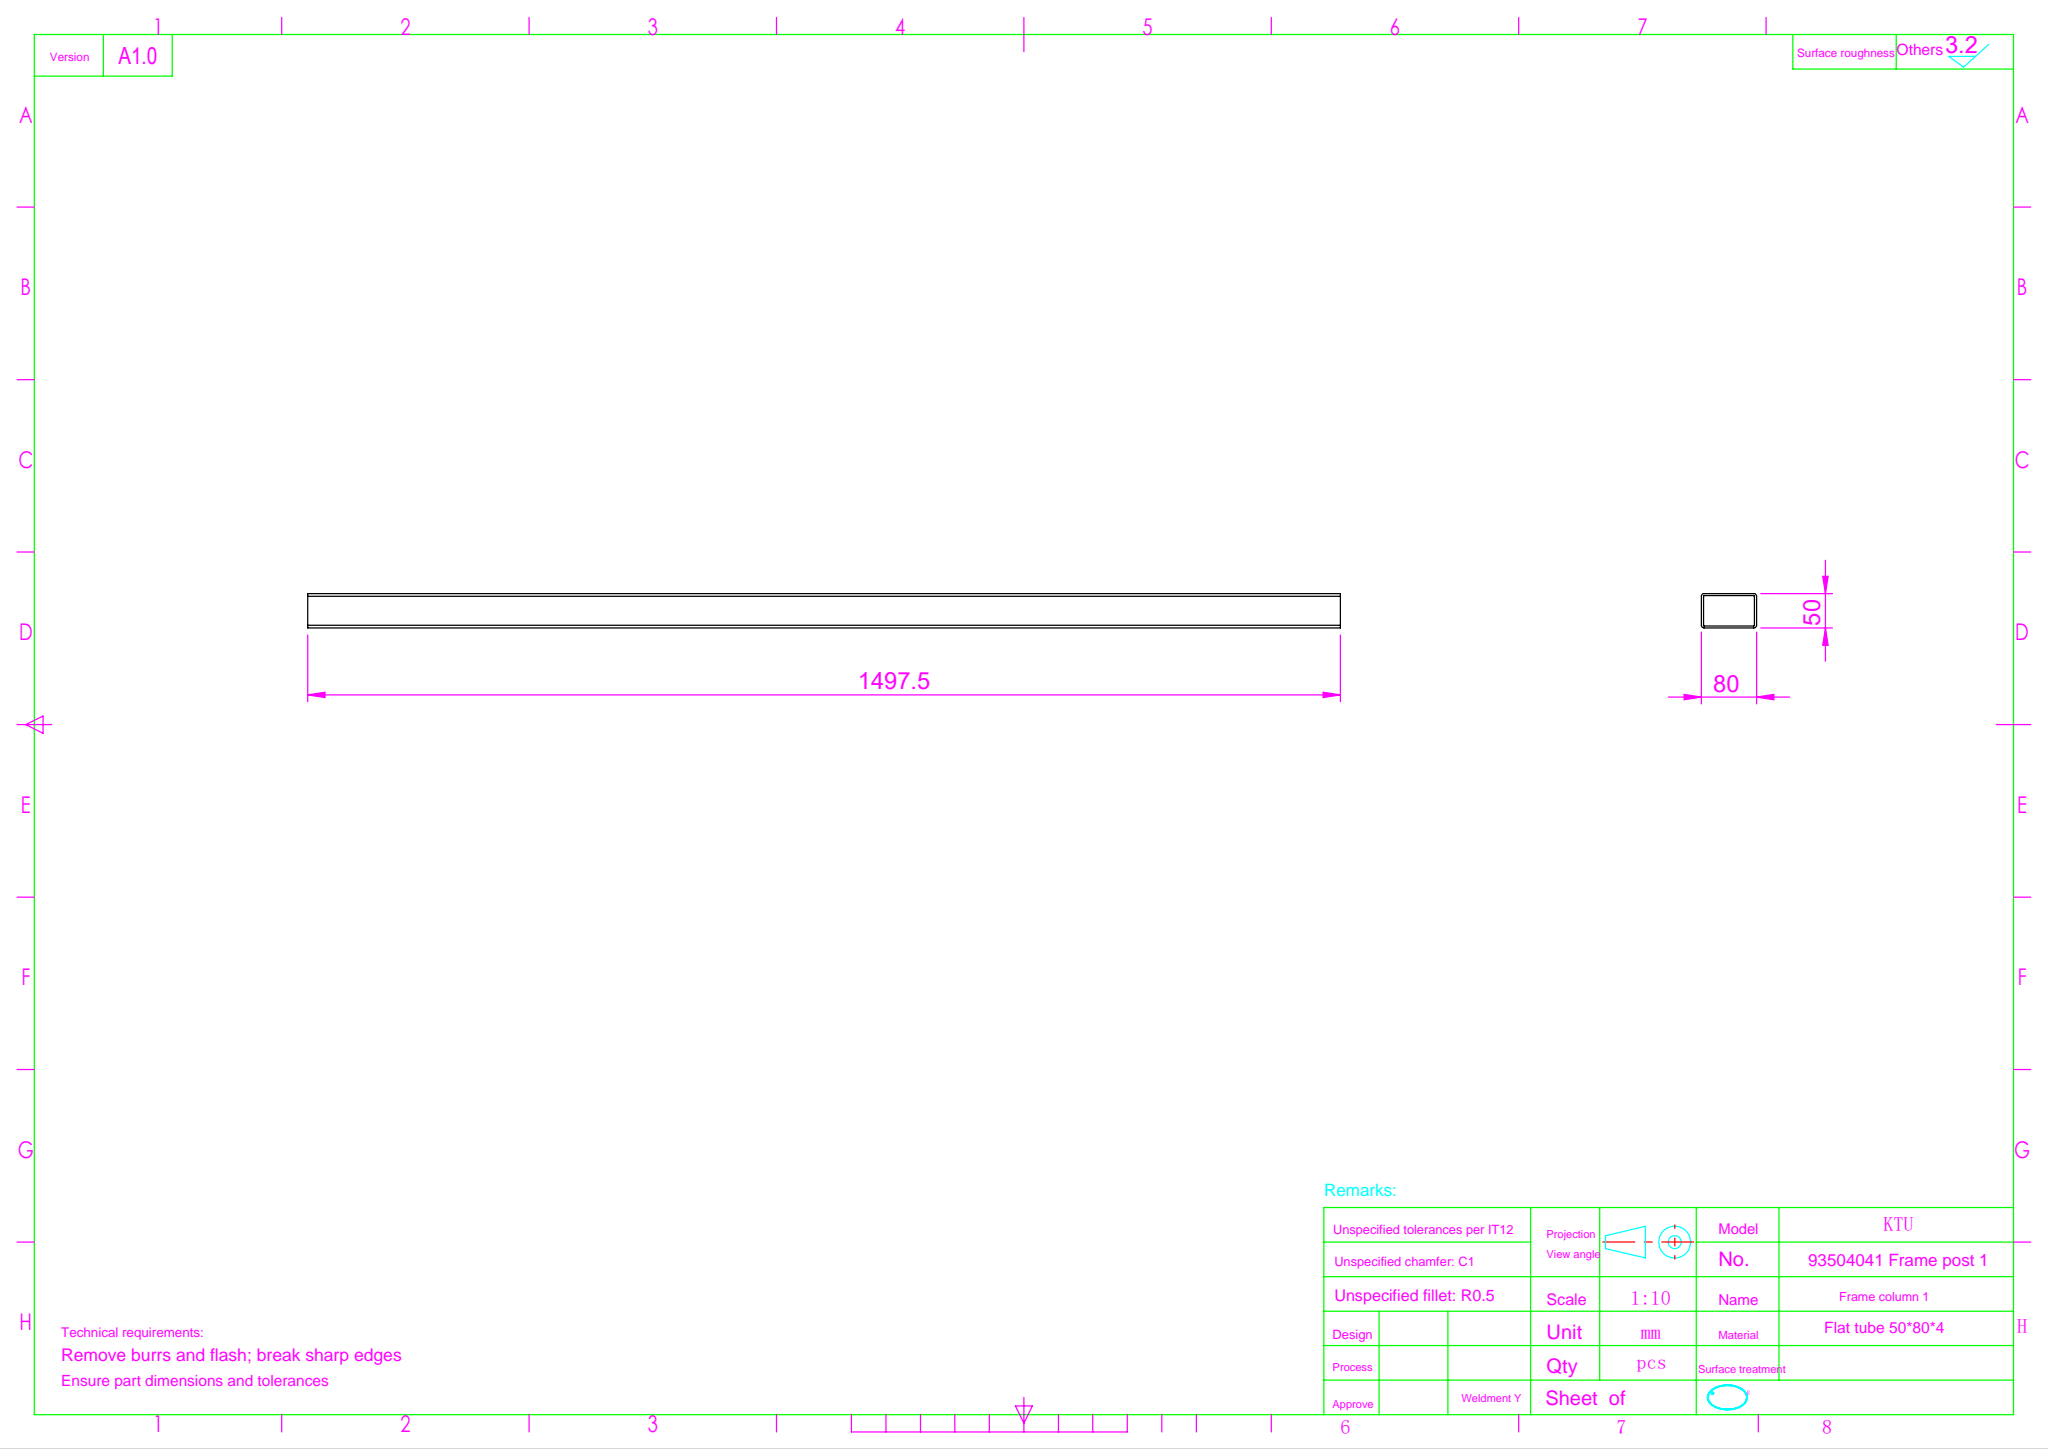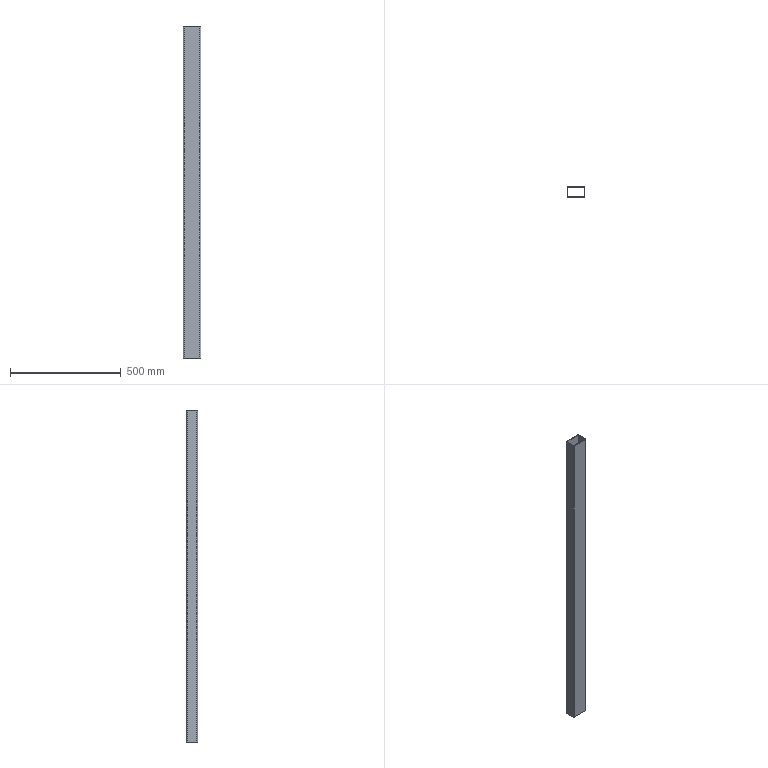Part | SolidWorks | features ExtruThin 1 | 1 solid | 18 faces | box 80 x 50 x 1498 mm | volume 1094858 mm3 | plane 10 | cylinder 8 | commonest cylinder face diameters 2 x4 8 x4
STEP:
#1=CARTESIAN_POINT('',(36.,-25.,748.75));
#2=VERTEX_POINT('',#1);
#3=CARTESIAN_POINT('',(40.,-21.,748.75));
#4=VERTEX_POINT('',#3);
#5=CARTESIAN_POINT('',(36.,-21.,748.75));
#6=DIRECTION('',(0.,0.,1.));
#7=DIRECTION('',(1.,0.,0.));
#8=AXIS2_PLACEMENT_3D('',#5,#6,#7);
#9=CIRCLE('',#8,4.);
#10=EDGE_CURVE('',#2,#4,#9,.T.);
#11=ORIENTED_EDGE('',*,*,#10,.T.);
#12=CARTESIAN_POINT('',(40.,21.,748.75));
#13=VERTEX_POINT('',#12);
#14=CARTESIAN_POINT('',(40.,21.,748.75));
#15=DIRECTION('',(0.,1.,0.));
#16=VECTOR('',#15,1000.);
#17=LINE('',#14,#16);
#18=EDGE_CURVE('',#4,#13,#17,.T.);
#19=ORIENTED_EDGE('',*,*,#18,.T.);
#20=CARTESIAN_POINT('',(36.,25.,748.75));
#21=VERTEX_POINT('',#20);
#22=CARTESIAN_POINT('',(36.,21.,748.75));
#23=DIRECTION('',(0.,0.,1.));
#24=DIRECTION('',(-1.,0.,0.));
#25=AXIS2_PLACEMENT_3D('',#22,#23,#24);
#26=CIRCLE('',#25,4.);
#27=EDGE_CURVE('',#13,#21,#26,.T.);
#28=ORIENTED_EDGE('',*,*,#27,.T.);
#29=CARTESIAN_POINT('',(-36.,25.,748.75));
#30=VERTEX_POINT('',#29);
#31=CARTESIAN_POINT('',(-36.,25.,748.75));
#32=DIRECTION('',(-1.,0.,0.));
#33=VECTOR('',#32,1000.);
#34=LINE('',#31,#33);
#35=EDGE_CURVE('',#21,#30,#34,.T.);
#36=ORIENTED_EDGE('',*,*,#35,.T.);
#37=CARTESIAN_POINT('',(-40.,21.,748.75));
#38=VERTEX_POINT('',#37);
#39=CARTESIAN_POINT('',(-36.,21.,748.75));
#40=DIRECTION('',(0.,0.,1.));
#41=DIRECTION('',(1.,0.,0.));
#42=AXIS2_PLACEMENT_3D('',#39,#40,#41);
#43=CIRCLE('',#42,4.);
#44=EDGE_CURVE('',#30,#38,#43,.T.);
#45=ORIENTED_EDGE('',*,*,#44,.T.);
#46=CARTESIAN_POINT('',(-40.,-21.,748.75));
#47=VERTEX_POINT('',#46);
#48=CARTESIAN_POINT('',(-40.,21.,748.75));
#49=DIRECTION('',(0.,-1.,0.));
#50=VECTOR('',#49,1000.);
#51=LINE('',#48,#50);
#52=EDGE_CURVE('',#38,#47,#51,.T.);
#53=ORIENTED_EDGE('',*,*,#52,.T.);
#54=CARTESIAN_POINT('',(-36.,-25.,748.75));
#55=VERTEX_POINT('',#54);
#56=CARTESIAN_POINT('',(-36.,-21.,748.75));
#57=DIRECTION('',(0.,0.,1.));
#58=DIRECTION('',(1.,0.,0.));
#59=AXIS2_PLACEMENT_3D('',#56,#57,#58);
#60=CIRCLE('',#59,4.);
#61=EDGE_CURVE('',#47,#55,#60,.T.);
#62=ORIENTED_EDGE('',*,*,#61,.T.);
#63=CARTESIAN_POINT('',(-36.,-25.,748.75));
#64=DIRECTION('',(1.,0.,0.));
#65=VECTOR('',#64,1000.);
#66=LINE('',#63,#65);
#67=EDGE_CURVE('',#55,#2,#66,.T.);
#68=ORIENTED_EDGE('',*,*,#67,.T.);
#69=EDGE_LOOP('',(#11,#19,#28,#36,#45,#53,#62,#68));
#70=FACE_OUTER_BOUND('',#69,.T.);
#71=CARTESIAN_POINT('',(37.,-21.,748.75));
#72=VERTEX_POINT('',#71);
#73=CARTESIAN_POINT('',(37.,21.,748.75));
#74=VERTEX_POINT('',#73);
#75=CARTESIAN_POINT('',(37.,21.,748.75));
#76=DIRECTION('',(0.,1.,0.));
#77=VECTOR('',#76,1000.);
#78=LINE('',#75,#77);
#79=EDGE_CURVE('',#72,#74,#78,.T.);
#80=ORIENTED_EDGE('',*,*,#79,.F.);
#81=CARTESIAN_POINT('',(36.,-22.,748.75));
#82=VERTEX_POINT('',#81);
#83=CARTESIAN_POINT('',(36.,-21.,748.75));
#84=DIRECTION('',(0.,0.,1.));
#85=DIRECTION('',(1.,0.,0.));
#86=AXIS2_PLACEMENT_3D('',#83,#84,#85);
#87=CIRCLE('',#86,1.);
#88=EDGE_CURVE('',#82,#72,#87,.T.);
#89=ORIENTED_EDGE('',*,*,#88,.F.);
#90=CARTESIAN_POINT('',(-36.,-22.,748.75));
#91=VERTEX_POINT('',#90);
#92=CARTESIAN_POINT('',(-36.,-22.,748.75));
#93=DIRECTION('',(1.,0.,0.));
#94=VECTOR('',#93,1000.);
#95=LINE('',#92,#94);
#96=EDGE_CURVE('',#91,#82,#95,.T.);
#97=ORIENTED_EDGE('',*,*,#96,.F.);
#98=CARTESIAN_POINT('',(-37.,-21.,748.75));
#99=VERTEX_POINT('',#98);
#100=CARTESIAN_POINT('',(-36.,-21.,748.75));
#101=DIRECTION('',(0.,0.,1.));
#102=DIRECTION('',(1.,0.,0.));
#103=AXIS2_PLACEMENT_3D('',#100,#101,#102);
#104=CIRCLE('',#103,1.);
#105=EDGE_CURVE('',#99,#91,#104,.T.);
#106=ORIENTED_EDGE('',*,*,#105,.F.);
#107=CARTESIAN_POINT('',(-37.,21.,748.75));
#108=VERTEX_POINT('',#107);
#109=CARTESIAN_POINT('',(-37.,21.,748.75));
#110=DIRECTION('',(0.,-1.,0.));
#111=VECTOR('',#110,1000.);
#112=LINE('',#109,#111);
#113=EDGE_CURVE('',#108,#99,#112,.T.);
#114=ORIENTED_EDGE('',*,*,#113,.F.);
#115=CARTESIAN_POINT('',(-36.,22.,748.75));
#116=VERTEX_POINT('',#115);
#117=CARTESIAN_POINT('',(-36.,21.,748.75));
#118=DIRECTION('',(0.,0.,1.));
#119=DIRECTION('',(1.,0.,0.));
#120=AXIS2_PLACEMENT_3D('',#117,#118,#119);
#121=CIRCLE('',#120,1.);
#122=EDGE_CURVE('',#116,#108,#121,.T.);
#123=ORIENTED_EDGE('',*,*,#122,.F.);
#124=CARTESIAN_POINT('',(36.,22.,748.75));
#125=VERTEX_POINT('',#124);
#126=CARTESIAN_POINT('',(-36.,22.,748.75));
#127=DIRECTION('',(-1.,0.,0.));
#128=VECTOR('',#127,1000.);
#129=LINE('',#126,#128);
#130=EDGE_CURVE('',#125,#116,#129,.T.);
#131=ORIENTED_EDGE('',*,*,#130,.F.);
#132=CARTESIAN_POINT('',(36.,21.,748.75));
#133=DIRECTION('',(0.,0.,1.));
#134=DIRECTION('',(1.,0.,0.));
#135=AXIS2_PLACEMENT_3D('',#132,#133,#134);
#136=CIRCLE('',#135,1.);
#137=EDGE_CURVE('',#74,#125,#136,.T.);
#138=ORIENTED_EDGE('',*,*,#137,.F.);
#139=EDGE_LOOP('',(#80,#89,#97,#106,#114,#123,#131,#138));
#140=FACE_BOUND('',#139,.T.);
#141=CARTESIAN_POINT('',(36.,-21.,748.75));
#142=DIRECTION('',(0.,0.,1.));
#143=DIRECTION('',(1.,0.,0.));
#144=AXIS2_PLACEMENT_3D('',#141,#142,#143);
#145=PLANE('',#144);
#146=ADVANCED_FACE('',(#70,#140),#145,.T.);
#147=CARTESIAN_POINT('',(36.,-25.,-748.75));
#148=VERTEX_POINT('',#147);
#149=CARTESIAN_POINT('',(40.,-21.,-748.75));
#150=VERTEX_POINT('',#149);
#151=CARTESIAN_POINT('',(36.,-21.,-748.75));
#152=DIRECTION('',(0.,0.,1.));
#153=DIRECTION('',(1.,0.,0.));
#154=AXIS2_PLACEMENT_3D('',#151,#152,#153);
#155=CIRCLE('',#154,4.);
#156=EDGE_CURVE('',#148,#150,#155,.T.);
#157=ORIENTED_EDGE('',*,*,#156,.F.);
#158=CARTESIAN_POINT('',(-36.,-25.,-748.75));
#159=VERTEX_POINT('',#158);
#160=CARTESIAN_POINT('',(-36.,-25.,-748.75));
#161=DIRECTION('',(1.,0.,0.));
#162=VECTOR('',#161,1000.);
#163=LINE('',#160,#162);
#164=EDGE_CURVE('',#159,#148,#163,.T.);
#165=ORIENTED_EDGE('',*,*,#164,.F.);
#166=CARTESIAN_POINT('',(-40.,-21.,-748.75));
#167=VERTEX_POINT('',#166);
#168=CARTESIAN_POINT('',(-36.,-21.,-748.75));
#169=DIRECTION('',(0.,0.,1.));
#170=DIRECTION('',(1.,0.,0.));
#171=AXIS2_PLACEMENT_3D('',#168,#169,#170);
#172=CIRCLE('',#171,4.);
#173=EDGE_CURVE('',#167,#159,#172,.T.);
#174=ORIENTED_EDGE('',*,*,#173,.F.);
#175=CARTESIAN_POINT('',(-40.,21.,-748.75));
#176=VERTEX_POINT('',#175);
#177=CARTESIAN_POINT('',(-40.,21.,-748.75));
#178=DIRECTION('',(0.,-1.,0.));
#179=VECTOR('',#178,1000.);
#180=LINE('',#177,#179);
#181=EDGE_CURVE('',#176,#167,#180,.T.);
#182=ORIENTED_EDGE('',*,*,#181,.F.);
#183=CARTESIAN_POINT('',(-36.,25.,-748.75));
#184=VERTEX_POINT('',#183);
#185=CARTESIAN_POINT('',(-36.,21.,-748.75));
#186=DIRECTION('',(0.,0.,1.));
#187=DIRECTION('',(1.,0.,0.));
#188=AXIS2_PLACEMENT_3D('',#185,#186,#187);
#189=CIRCLE('',#188,4.);
#190=EDGE_CURVE('',#184,#176,#189,.T.);
#191=ORIENTED_EDGE('',*,*,#190,.F.);
#192=CARTESIAN_POINT('',(36.,25.,-748.75));
#193=VERTEX_POINT('',#192);
#194=CARTESIAN_POINT('',(-36.,25.,-748.75));
#195=DIRECTION('',(-1.,0.,0.));
#196=VECTOR('',#195,1000.);
#197=LINE('',#194,#196);
#198=EDGE_CURVE('',#193,#184,#197,.T.);
#199=ORIENTED_EDGE('',*,*,#198,.F.);
#200=CARTESIAN_POINT('',(40.,21.,-748.75));
#201=VERTEX_POINT('',#200);
#202=CARTESIAN_POINT('',(36.,21.,-748.75));
#203=DIRECTION('',(0.,0.,1.));
#204=DIRECTION('',(-1.,0.,0.));
#205=AXIS2_PLACEMENT_3D('',#202,#203,#204);
#206=CIRCLE('',#205,4.);
#207=EDGE_CURVE('',#201,#193,#206,.T.);
#208=ORIENTED_EDGE('',*,*,#207,.F.);
#209=CARTESIAN_POINT('',(40.,21.,-748.75));
#210=DIRECTION('',(0.,1.,0.));
#211=VECTOR('',#210,1000.);
#212=LINE('',#209,#211);
#213=EDGE_CURVE('',#150,#201,#212,.T.);
#214=ORIENTED_EDGE('',*,*,#213,.F.);
#215=EDGE_LOOP('',(#157,#165,#174,#182,#191,#199,#208,#214));
#216=FACE_OUTER_BOUND('',#215,.T.);
#217=CARTESIAN_POINT('',(36.,-22.,-748.75));
#218=VERTEX_POINT('',#217);
#219=CARTESIAN_POINT('',(37.,-21.,-748.75));
#220=VERTEX_POINT('',#219);
#221=CARTESIAN_POINT('',(36.,-21.,-748.75));
#222=DIRECTION('',(0.,0.,1.));
#223=DIRECTION('',(1.,0.,0.));
#224=AXIS2_PLACEMENT_3D('',#221,#222,#223);
#225=CIRCLE('',#224,1.);
#226=EDGE_CURVE('',#218,#220,#225,.T.);
#227=ORIENTED_EDGE('',*,*,#226,.T.);
#228=CARTESIAN_POINT('',(37.,21.,-748.75));
#229=VERTEX_POINT('',#228);
#230=CARTESIAN_POINT('',(37.,21.,-748.75));
#231=DIRECTION('',(0.,1.,0.));
#232=VECTOR('',#231,1000.);
#233=LINE('',#230,#232);
#234=EDGE_CURVE('',#220,#229,#233,.T.);
#235=ORIENTED_EDGE('',*,*,#234,.T.);
#236=CARTESIAN_POINT('',(36.,22.,-748.75));
#237=VERTEX_POINT('',#236);
#238=CARTESIAN_POINT('',(36.,21.,-748.75));
#239=DIRECTION('',(0.,0.,1.));
#240=DIRECTION('',(1.,0.,0.));
#241=AXIS2_PLACEMENT_3D('',#238,#239,#240);
#242=CIRCLE('',#241,1.);
#243=EDGE_CURVE('',#229,#237,#242,.T.);
#244=ORIENTED_EDGE('',*,*,#243,.T.);
#245=CARTESIAN_POINT('',(-36.,22.,-748.75));
#246=VERTEX_POINT('',#245);
#247=CARTESIAN_POINT('',(-36.,22.,-748.75));
#248=DIRECTION('',(-1.,0.,0.));
#249=VECTOR('',#248,1000.);
#250=LINE('',#247,#249);
#251=EDGE_CURVE('',#237,#246,#250,.T.);
#252=ORIENTED_EDGE('',*,*,#251,.T.);
#253=CARTESIAN_POINT('',(-37.,21.,-748.75));
#254=VERTEX_POINT('',#253);
#255=CARTESIAN_POINT('',(-36.,21.,-748.75));
#256=DIRECTION('',(0.,0.,1.));
#257=DIRECTION('',(1.,0.,0.));
#258=AXIS2_PLACEMENT_3D('',#255,#256,#257);
#259=CIRCLE('',#258,1.);
#260=EDGE_CURVE('',#246,#254,#259,.T.);
#261=ORIENTED_EDGE('',*,*,#260,.T.);
#262=CARTESIAN_POINT('',(-37.,-21.,-748.75));
#263=VERTEX_POINT('',#262);
#264=CARTESIAN_POINT('',(-37.,21.,-748.75));
#265=DIRECTION('',(0.,-1.,0.));
#266=VECTOR('',#265,1000.);
#267=LINE('',#264,#266);
#268=EDGE_CURVE('',#254,#263,#267,.T.);
#269=ORIENTED_EDGE('',*,*,#268,.T.);
#270=CARTESIAN_POINT('',(-36.,-22.,-748.75));
#271=VERTEX_POINT('',#270);
#272=CARTESIAN_POINT('',(-36.,-21.,-748.75));
#273=DIRECTION('',(0.,0.,1.));
#274=DIRECTION('',(1.,0.,0.));
#275=AXIS2_PLACEMENT_3D('',#272,#273,#274);
#276=CIRCLE('',#275,1.);
#277=EDGE_CURVE('',#263,#271,#276,.T.);
#278=ORIENTED_EDGE('',*,*,#277,.T.);
#279=CARTESIAN_POINT('',(-36.,-22.,-748.75));
#280=DIRECTION('',(1.,0.,0.));
#281=VECTOR('',#280,1000.);
#282=LINE('',#279,#281);
#283=EDGE_CURVE('',#271,#218,#282,.T.);
#284=ORIENTED_EDGE('',*,*,#283,.T.);
#285=EDGE_LOOP('',(#227,#235,#244,#252,#261,#269,#278,#284));
#286=FACE_BOUND('',#285,.T.);
#287=CARTESIAN_POINT('',(36.,-21.,-748.75));
#288=DIRECTION('',(0.,0.,1.));
#289=DIRECTION('',(1.,0.,0.));
#290=AXIS2_PLACEMENT_3D('',#287,#288,#289);
#291=PLANE('',#290);
#292=ADVANCED_FACE('',(#216,#286),#291,.F.);
#293=ORIENTED_EDGE('',*,*,#156,.T.);
#294=CARTESIAN_POINT('',(40.,-21.,748.75));
#295=DIRECTION('',(0.,0.,-1.));
#296=VECTOR('',#295,1000.);
#297=LINE('',#294,#296);
#298=EDGE_CURVE('',#4,#150,#297,.T.);
#299=ORIENTED_EDGE('',*,*,#298,.F.);
#300=ORIENTED_EDGE('',*,*,#10,.F.);
#301=CARTESIAN_POINT('',(36.,-25.,748.75));
#302=DIRECTION('',(0.,0.,-1.));
#303=VECTOR('',#302,1000.);
#304=LINE('',#301,#303);
#305=EDGE_CURVE('',#2,#148,#304,.T.);
#306=ORIENTED_EDGE('',*,*,#305,.T.);
#307=EDGE_LOOP('',(#293,#299,#300,#306));
#308=FACE_OUTER_BOUND('',#307,.T.);
#309=CARTESIAN_POINT('',(36.,-21.,748.75));
#310=DIRECTION('',(0.,0.,-1.));
#311=DIRECTION('',(-1.,0.,0.));
#312=AXIS2_PLACEMENT_3D('',#309,#310,#311);
#313=CYLINDRICAL_SURFACE('',#312,4.);
#314=ADVANCED_FACE('',(#308),#313,.T.);
#315=ORIENTED_EDGE('',*,*,#213,.T.);
#316=CARTESIAN_POINT('',(40.,21.,748.75));
#317=DIRECTION('',(0.,0.,-1.));
#318=VECTOR('',#317,1000.);
#319=LINE('',#316,#318);
#320=EDGE_CURVE('',#13,#201,#319,.T.);
#321=ORIENTED_EDGE('',*,*,#320,.F.);
#322=ORIENTED_EDGE('',*,*,#18,.F.);
#323=ORIENTED_EDGE('',*,*,#298,.T.);
#324=EDGE_LOOP('',(#315,#321,#322,#323));
#325=FACE_OUTER_BOUND('',#324,.T.);
#326=CARTESIAN_POINT('',(40.,21.,748.75));
#327=DIRECTION('',(-1.,0.,0.));
#328=DIRECTION('',(0.,-1.,0.));
#329=AXIS2_PLACEMENT_3D('',#326,#327,#328);
#330=PLANE('',#329);
#331=ADVANCED_FACE('',(#325),#330,.F.);
#332=ORIENTED_EDGE('',*,*,#207,.T.);
#333=CARTESIAN_POINT('',(36.,25.,748.75));
#334=DIRECTION('',(0.,0.,-1.));
#335=VECTOR('',#334,1000.);
#336=LINE('',#333,#335);
#337=EDGE_CURVE('',#21,#193,#336,.T.);
#338=ORIENTED_EDGE('',*,*,#337,.F.);
#339=ORIENTED_EDGE('',*,*,#27,.F.);
#340=ORIENTED_EDGE('',*,*,#320,.T.);
#341=EDGE_LOOP('',(#332,#338,#339,#340));
#342=FACE_OUTER_BOUND('',#341,.T.);
#343=CARTESIAN_POINT('',(36.,21.,748.75));
#344=DIRECTION('',(0.,0.,-1.));
#345=DIRECTION('',(-1.,0.,0.));
#346=AXIS2_PLACEMENT_3D('',#343,#344,#345);
#347=CYLINDRICAL_SURFACE('',#346,4.);
#348=ADVANCED_FACE('',(#342),#347,.T.);
#349=ORIENTED_EDGE('',*,*,#198,.T.);
#350=CARTESIAN_POINT('',(-36.,25.,748.75));
#351=DIRECTION('',(0.,0.,-1.));
#352=VECTOR('',#351,1000.);
#353=LINE('',#350,#352);
#354=EDGE_CURVE('',#30,#184,#353,.T.);
#355=ORIENTED_EDGE('',*,*,#354,.F.);
#356=ORIENTED_EDGE('',*,*,#35,.F.);
#357=ORIENTED_EDGE('',*,*,#337,.T.);
#358=EDGE_LOOP('',(#349,#355,#356,#357));
#359=FACE_OUTER_BOUND('',#358,.T.);
#360=CARTESIAN_POINT('',(-36.,25.,748.75));
#361=DIRECTION('',(0.,-1.,0.));
#362=DIRECTION('',(0.,0.,-1.));
#363=AXIS2_PLACEMENT_3D('',#360,#361,#362);
#364=PLANE('',#363);
#365=ADVANCED_FACE('',(#359),#364,.F.);
#366=ORIENTED_EDGE('',*,*,#190,.T.);
#367=CARTESIAN_POINT('',(-40.,21.,748.75));
#368=DIRECTION('',(0.,0.,-1.));
#369=VECTOR('',#368,1000.);
#370=LINE('',#367,#369);
#371=EDGE_CURVE('',#38,#176,#370,.T.);
#372=ORIENTED_EDGE('',*,*,#371,.F.);
#373=ORIENTED_EDGE('',*,*,#44,.F.);
#374=ORIENTED_EDGE('',*,*,#354,.T.);
#375=EDGE_LOOP('',(#366,#372,#373,#374));
#376=FACE_OUTER_BOUND('',#375,.T.);
#377=CARTESIAN_POINT('',(-36.,21.,748.75));
#378=DIRECTION('',(0.,0.,-1.));
#379=DIRECTION('',(-1.,0.,0.));
#380=AXIS2_PLACEMENT_3D('',#377,#378,#379);
#381=CYLINDRICAL_SURFACE('',#380,4.);
#382=ADVANCED_FACE('',(#376),#381,.T.);
#383=ORIENTED_EDGE('',*,*,#181,.T.);
#384=CARTESIAN_POINT('',(-40.,-21.,748.75));
#385=DIRECTION('',(0.,0.,-1.));
#386=VECTOR('',#385,1000.);
#387=LINE('',#384,#386);
#388=EDGE_CURVE('',#47,#167,#387,.T.);
#389=ORIENTED_EDGE('',*,*,#388,.F.);
#390=ORIENTED_EDGE('',*,*,#52,.F.);
#391=ORIENTED_EDGE('',*,*,#371,.T.);
#392=EDGE_LOOP('',(#383,#389,#390,#391));
#393=FACE_OUTER_BOUND('',#392,.T.);
#394=CARTESIAN_POINT('',(-40.,21.,748.75));
#395=DIRECTION('',(1.,0.,0.));
#396=DIRECTION('',(0.,1.,0.));
#397=AXIS2_PLACEMENT_3D('',#394,#395,#396);
#398=PLANE('',#397);
#399=ADVANCED_FACE('',(#393),#398,.F.);
#400=ORIENTED_EDGE('',*,*,#173,.T.);
#401=CARTESIAN_POINT('',(-36.,-25.,748.75));
#402=DIRECTION('',(0.,0.,-1.));
#403=VECTOR('',#402,1000.);
#404=LINE('',#401,#403);
#405=EDGE_CURVE('',#55,#159,#404,.T.);
#406=ORIENTED_EDGE('',*,*,#405,.F.);
#407=ORIENTED_EDGE('',*,*,#61,.F.);
#408=ORIENTED_EDGE('',*,*,#388,.T.);
#409=EDGE_LOOP('',(#400,#406,#407,#408));
#410=FACE_OUTER_BOUND('',#409,.T.);
#411=CARTESIAN_POINT('',(-36.,-21.,748.75));
#412=DIRECTION('',(0.,0.,-1.));
#413=DIRECTION('',(-1.,0.,0.));
#414=AXIS2_PLACEMENT_3D('',#411,#412,#413);
#415=CYLINDRICAL_SURFACE('',#414,4.);
#416=ADVANCED_FACE('',(#410),#415,.T.);
#417=ORIENTED_EDGE('',*,*,#164,.T.);
#418=ORIENTED_EDGE('',*,*,#305,.F.);
#419=ORIENTED_EDGE('',*,*,#67,.F.);
#420=ORIENTED_EDGE('',*,*,#405,.T.);
#421=EDGE_LOOP('',(#417,#418,#419,#420));
#422=FACE_OUTER_BOUND('',#421,.T.);
#423=CARTESIAN_POINT('',(-36.,-25.,748.75));
#424=DIRECTION('',(0.,1.,0.));
#425=DIRECTION('',(0.,0.,1.));
#426=AXIS2_PLACEMENT_3D('',#423,#424,#425);
#427=PLANE('',#426);
#428=ADVANCED_FACE('',(#422),#427,.F.);
#429=ORIENTED_EDGE('',*,*,#226,.F.);
#430=CARTESIAN_POINT('',(36.,-22.,748.75));
#431=DIRECTION('',(0.,0.,-1.));
#432=VECTOR('',#431,1000.);
#433=LINE('',#430,#432);
#434=EDGE_CURVE('',#82,#218,#433,.T.);
#435=ORIENTED_EDGE('',*,*,#434,.F.);
#436=ORIENTED_EDGE('',*,*,#88,.T.);
#437=CARTESIAN_POINT('',(37.,-21.,748.75));
#438=DIRECTION('',(0.,0.,-1.));
#439=VECTOR('',#438,1000.);
#440=LINE('',#437,#439);
#441=EDGE_CURVE('',#72,#220,#440,.T.);
#442=ORIENTED_EDGE('',*,*,#441,.T.);
#443=EDGE_LOOP('',(#429,#435,#436,#442));
#444=FACE_OUTER_BOUND('',#443,.T.);
#445=CARTESIAN_POINT('',(36.,-21.,748.75));
#446=DIRECTION('',(0.,0.,-1.));
#447=DIRECTION('',(-1.,0.,0.));
#448=AXIS2_PLACEMENT_3D('',#445,#446,#447);
#449=CYLINDRICAL_SURFACE('',#448,1.);
#450=ADVANCED_FACE('',(#444),#449,.F.);
#451=ORIENTED_EDGE('',*,*,#234,.F.);
#452=ORIENTED_EDGE('',*,*,#441,.F.);
#453=ORIENTED_EDGE('',*,*,#79,.T.);
#454=CARTESIAN_POINT('',(37.,21.,748.75));
#455=DIRECTION('',(0.,0.,-1.));
#456=VECTOR('',#455,1000.);
#457=LINE('',#454,#456);
#458=EDGE_CURVE('',#74,#229,#457,.T.);
#459=ORIENTED_EDGE('',*,*,#458,.T.);
#460=EDGE_LOOP('',(#451,#452,#453,#459));
#461=FACE_OUTER_BOUND('',#460,.T.);
#462=CARTESIAN_POINT('',(37.,21.,748.75));
#463=DIRECTION('',(-1.,0.,0.));
#464=DIRECTION('',(0.,-1.,0.));
#465=AXIS2_PLACEMENT_3D('',#462,#463,#464);
#466=PLANE('',#465);
#467=ADVANCED_FACE('',(#461),#466,.T.);
#468=ORIENTED_EDGE('',*,*,#243,.F.);
#469=ORIENTED_EDGE('',*,*,#458,.F.);
#470=ORIENTED_EDGE('',*,*,#137,.T.);
#471=CARTESIAN_POINT('',(36.,22.,748.75));
#472=DIRECTION('',(0.,0.,-1.));
#473=VECTOR('',#472,1000.);
#474=LINE('',#471,#473);
#475=EDGE_CURVE('',#125,#237,#474,.T.);
#476=ORIENTED_EDGE('',*,*,#475,.T.);
#477=EDGE_LOOP('',(#468,#469,#470,#476));
#478=FACE_OUTER_BOUND('',#477,.T.);
#479=CARTESIAN_POINT('',(36.,21.,748.75));
#480=DIRECTION('',(0.,0.,-1.));
#481=DIRECTION('',(-1.,0.,0.));
#482=AXIS2_PLACEMENT_3D('',#479,#480,#481);
#483=CYLINDRICAL_SURFACE('',#482,1.);
#484=ADVANCED_FACE('',(#478),#483,.F.);
#485=ORIENTED_EDGE('',*,*,#251,.F.);
#486=ORIENTED_EDGE('',*,*,#475,.F.);
#487=ORIENTED_EDGE('',*,*,#130,.T.);
#488=CARTESIAN_POINT('',(-36.,22.,748.75));
#489=DIRECTION('',(0.,0.,-1.));
#490=VECTOR('',#489,1000.);
#491=LINE('',#488,#490);
#492=EDGE_CURVE('',#116,#246,#491,.T.);
#493=ORIENTED_EDGE('',*,*,#492,.T.);
#494=EDGE_LOOP('',(#485,#486,#487,#493));
#495=FACE_OUTER_BOUND('',#494,.T.);
#496=CARTESIAN_POINT('',(-36.,22.,748.75));
#497=DIRECTION('',(0.,-1.,0.));
#498=DIRECTION('',(0.,0.,-1.));
#499=AXIS2_PLACEMENT_3D('',#496,#497,#498);
#500=PLANE('',#499);
#501=ADVANCED_FACE('',(#495),#500,.T.);
#502=ORIENTED_EDGE('',*,*,#260,.F.);
#503=ORIENTED_EDGE('',*,*,#492,.F.);
#504=ORIENTED_EDGE('',*,*,#122,.T.);
#505=CARTESIAN_POINT('',(-37.,21.,748.75));
#506=DIRECTION('',(0.,0.,-1.));
#507=VECTOR('',#506,1000.);
#508=LINE('',#505,#507);
#509=EDGE_CURVE('',#108,#254,#508,.T.);
#510=ORIENTED_EDGE('',*,*,#509,.T.);
#511=EDGE_LOOP('',(#502,#503,#504,#510));
#512=FACE_OUTER_BOUND('',#511,.T.);
#513=CARTESIAN_POINT('',(-36.,21.,748.75));
#514=DIRECTION('',(0.,0.,-1.));
#515=DIRECTION('',(-1.,0.,0.));
#516=AXIS2_PLACEMENT_3D('',#513,#514,#515);
#517=CYLINDRICAL_SURFACE('',#516,1.);
#518=ADVANCED_FACE('',(#512),#517,.F.);
#519=ORIENTED_EDGE('',*,*,#268,.F.);
#520=ORIENTED_EDGE('',*,*,#509,.F.);
#521=ORIENTED_EDGE('',*,*,#113,.T.);
#522=CARTESIAN_POINT('',(-37.,-21.,748.75));
#523=DIRECTION('',(0.,0.,-1.));
#524=VECTOR('',#523,1000.);
#525=LINE('',#522,#524);
#526=EDGE_CURVE('',#99,#263,#525,.T.);
#527=ORIENTED_EDGE('',*,*,#526,.T.);
#528=EDGE_LOOP('',(#519,#520,#521,#527));
#529=FACE_OUTER_BOUND('',#528,.T.);
#530=CARTESIAN_POINT('',(-37.,21.,748.75));
#531=DIRECTION('',(1.,0.,0.));
#532=DIRECTION('',(0.,1.,0.));
#533=AXIS2_PLACEMENT_3D('',#530,#531,#532);
#534=PLANE('',#533);
#535=ADVANCED_FACE('',(#529),#534,.T.);
#536=ORIENTED_EDGE('',*,*,#277,.F.);
#537=ORIENTED_EDGE('',*,*,#526,.F.);
#538=ORIENTED_EDGE('',*,*,#105,.T.);
#539=CARTESIAN_POINT('',(-36.,-22.,748.75));
#540=DIRECTION('',(0.,0.,-1.));
#541=VECTOR('',#540,1000.);
#542=LINE('',#539,#541);
#543=EDGE_CURVE('',#91,#271,#542,.T.);
#544=ORIENTED_EDGE('',*,*,#543,.T.);
#545=EDGE_LOOP('',(#536,#537,#538,#544));
#546=FACE_OUTER_BOUND('',#545,.T.);
#547=CARTESIAN_POINT('',(-36.,-21.,748.75));
#548=DIRECTION('',(0.,0.,-1.));
#549=DIRECTION('',(-1.,0.,0.));
#550=AXIS2_PLACEMENT_3D('',#547,#548,#549);
#551=CYLINDRICAL_SURFACE('',#550,1.);
#552=ADVANCED_FACE('',(#546),#551,.F.);
#553=ORIENTED_EDGE('',*,*,#283,.F.);
#554=ORIENTED_EDGE('',*,*,#543,.F.);
#555=ORIENTED_EDGE('',*,*,#96,.T.);
#556=ORIENTED_EDGE('',*,*,#434,.T.);
#557=EDGE_LOOP('',(#553,#554,#555,#556));
#558=FACE_OUTER_BOUND('',#557,.T.);
#559=CARTESIAN_POINT('',(-36.,-22.,748.75));
#560=DIRECTION('',(0.,1.,0.));
#561=DIRECTION('',(0.,0.,1.));
#562=AXIS2_PLACEMENT_3D('',#559,#560,#561);
#563=PLANE('',#562);
#564=ADVANCED_FACE('',(#558),#563,.T.);
#565=CLOSED_SHELL('',(#146,#292,#314,#331,#348,#365,#382,#399,#416,#428,#450,#467,#484,#501,#518,#535,#552,#564));
#566=MANIFOLD_SOLID_BREP('',#565);
#567=CARTESIAN_POINT('',(0.,0.,0.));
#568=DIRECTION('',(0.,0.,1.));
#569=DIRECTION('',(1.,0.,0.));
#570=AXIS2_PLACEMENT_3D('',#567,#568,#569);
#571=(LENGTH_UNIT()NAMED_UNIT(*)SI_UNIT(.MILLI.,.METRE.));
#572=UNCERTAINTY_MEASURE_WITH_UNIT(LENGTH_MEASURE(0.00001),#571,'','');
#573=(NAMED_UNIT(*)PLANE_ANGLE_UNIT()SI_UNIT($,.RADIAN.));
#574=(NAMED_UNIT(*)SI_UNIT($,.STERADIAN.)SOLID_ANGLE_UNIT());
#575=(GEOMETRIC_REPRESENTATION_CONTEXT(3)GLOBAL_UNCERTAINTY_ASSIGNED_CONTEXT((#572))GLOBAL_UNIT_ASSIGNED_CONTEXT((#571,#573,#574))REPRESENTATION_CONTEXT('',''));
#576=ADVANCED_BREP_SHAPE_REPRESENTATION('',(#566,#570),#575);